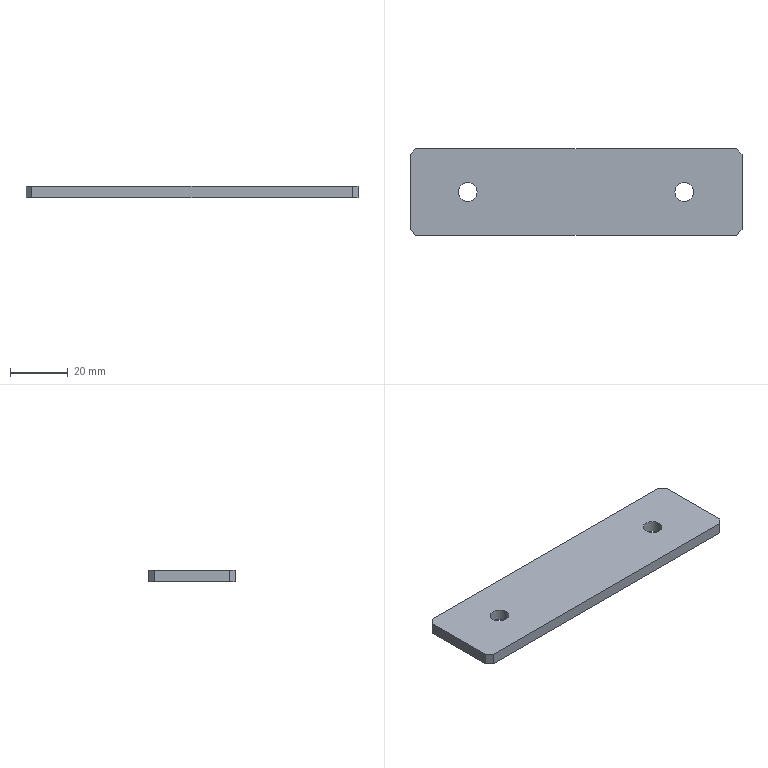Part | SolidWorks | features Chamfer 1, Extrusion 1 | 1 solid | 14 faces | box 115 x 30 x 4 mm | volume 13503 mm3 | plane 10 | cylinder 4 | commonest cylinder face diameters 6.5 x4
STEP:
#1=CARTESIAN_POINT('',(34.25,0.,4.));
#2=VERTEX_POINT('',#1);
#3=CARTESIAN_POINT('',(40.75,0.,4.));
#4=VERTEX_POINT('',#3);
#5=CARTESIAN_POINT('',(37.5,0.,4.));
#6=DIRECTION('',(0.,0.,1.));
#7=DIRECTION('',(1.,0.,0.));
#8=AXIS2_PLACEMENT_3D('',#5,#6,#7);
#9=CIRCLE('',#8,3.25);
#10=EDGE_CURVE('',#2,#4,#9,.T.);
#11=ORIENTED_EDGE('',*,*,#10,.T.);
#12=CARTESIAN_POINT('',(40.75,0.,0.));
#13=VERTEX_POINT('',#12);
#14=CARTESIAN_POINT('',(40.75,0.,4.));
#15=DIRECTION('',(0.,0.,-1.));
#16=VECTOR('',#15,1000.);
#17=LINE('',#14,#16);
#18=EDGE_CURVE('',#4,#13,#17,.T.);
#19=ORIENTED_EDGE('',*,*,#18,.T.);
#20=CARTESIAN_POINT('',(34.25,0.,0.));
#21=VERTEX_POINT('',#20);
#22=CARTESIAN_POINT('',(37.5,0.,0.));
#23=DIRECTION('',(0.,0.,1.));
#24=DIRECTION('',(1.,0.,0.));
#25=AXIS2_PLACEMENT_3D('',#22,#23,#24);
#26=CIRCLE('',#25,3.25);
#27=EDGE_CURVE('',#21,#13,#26,.T.);
#28=ORIENTED_EDGE('',*,*,#27,.F.);
#29=CARTESIAN_POINT('',(34.25,0.,4.));
#30=DIRECTION('',(0.,0.,-1.));
#31=VECTOR('',#30,1000.);
#32=LINE('',#29,#31);
#33=EDGE_CURVE('',#2,#21,#32,.T.);
#34=ORIENTED_EDGE('',*,*,#33,.F.);
#35=EDGE_LOOP('',(#11,#19,#28,#34));
#36=FACE_OUTER_BOUND('',#35,.T.);
#37=CARTESIAN_POINT('',(37.5,0.,4.));
#38=DIRECTION('',(0.,0.,-1.));
#39=DIRECTION('',(-1.,0.,0.));
#40=AXIS2_PLACEMENT_3D('',#37,#38,#39);
#41=CYLINDRICAL_SURFACE('',#40,3.25);
#42=ADVANCED_FACE('',(#36),#41,.F.);
#43=CARTESIAN_POINT('',(-40.75,0.,4.));
#44=VERTEX_POINT('',#43);
#45=CARTESIAN_POINT('',(-34.25,0.,4.));
#46=VERTEX_POINT('',#45);
#47=CARTESIAN_POINT('',(-37.5,0.,4.));
#48=DIRECTION('',(0.,0.,1.));
#49=DIRECTION('',(1.,0.,0.));
#50=AXIS2_PLACEMENT_3D('',#47,#48,#49);
#51=CIRCLE('',#50,3.25);
#52=EDGE_CURVE('',#44,#46,#51,.T.);
#53=ORIENTED_EDGE('',*,*,#52,.T.);
#54=CARTESIAN_POINT('',(-34.25,0.,0.));
#55=VERTEX_POINT('',#54);
#56=CARTESIAN_POINT('',(-34.25,0.,4.));
#57=DIRECTION('',(0.,0.,-1.));
#58=VECTOR('',#57,1000.);
#59=LINE('',#56,#58);
#60=EDGE_CURVE('',#46,#55,#59,.T.);
#61=ORIENTED_EDGE('',*,*,#60,.T.);
#62=CARTESIAN_POINT('',(-40.75,0.,0.));
#63=VERTEX_POINT('',#62);
#64=CARTESIAN_POINT('',(-37.5,0.,0.));
#65=DIRECTION('',(0.,0.,1.));
#66=DIRECTION('',(1.,0.,0.));
#67=AXIS2_PLACEMENT_3D('',#64,#65,#66);
#68=CIRCLE('',#67,3.25);
#69=EDGE_CURVE('',#63,#55,#68,.T.);
#70=ORIENTED_EDGE('',*,*,#69,.F.);
#71=CARTESIAN_POINT('',(-40.75,0.,4.));
#72=DIRECTION('',(0.,0.,-1.));
#73=VECTOR('',#72,1000.);
#74=LINE('',#71,#73);
#75=EDGE_CURVE('',#44,#63,#74,.T.);
#76=ORIENTED_EDGE('',*,*,#75,.F.);
#77=EDGE_LOOP('',(#53,#61,#70,#76));
#78=FACE_OUTER_BOUND('',#77,.T.);
#79=CARTESIAN_POINT('',(-37.5,0.,4.));
#80=DIRECTION('',(0.,0.,-1.));
#81=DIRECTION('',(-1.,0.,0.));
#82=AXIS2_PLACEMENT_3D('',#79,#80,#81);
#83=CYLINDRICAL_SURFACE('',#82,3.25);
#84=ADVANCED_FACE('',(#78),#83,.F.);
#85=CARTESIAN_POINT('',(-57.5,13.,4.));
#86=VERTEX_POINT('',#85);
#87=CARTESIAN_POINT('',(-57.5,-13.,4.));
#88=VERTEX_POINT('',#87);
#89=CARTESIAN_POINT('',(-57.5,15.,4.));
#90=DIRECTION('',(0.,-1.,0.));
#91=VECTOR('',#90,1000.);
#92=LINE('',#89,#91);
#93=EDGE_CURVE('',#86,#88,#92,.T.);
#94=ORIENTED_EDGE('',*,*,#93,.T.);
#95=CARTESIAN_POINT('',(-55.5,-15.,4.));
#96=VERTEX_POINT('',#95);
#97=CARTESIAN_POINT('',(-55.5,-15.,4.));
#98=DIRECTION('',(0.7071,-0.7071,0.));
#99=VECTOR('',#98,1000.);
#100=LINE('',#97,#99);
#101=EDGE_CURVE('',#88,#96,#100,.T.);
#102=ORIENTED_EDGE('',*,*,#101,.T.);
#103=CARTESIAN_POINT('',(55.5,-15.,4.));
#104=VERTEX_POINT('',#103);
#105=CARTESIAN_POINT('',(57.5,-15.,4.));
#106=DIRECTION('',(1.,0.,0.));
#107=VECTOR('',#106,1000.);
#108=LINE('',#105,#107);
#109=EDGE_CURVE('',#96,#104,#108,.T.);
#110=ORIENTED_EDGE('',*,*,#109,.T.);
#111=CARTESIAN_POINT('',(57.5,-13.,4.));
#112=VERTEX_POINT('',#111);
#113=CARTESIAN_POINT('',(57.5,-13.,4.));
#114=DIRECTION('',(0.7071,0.7071,0.));
#115=VECTOR('',#114,1000.);
#116=LINE('',#113,#115);
#117=EDGE_CURVE('',#104,#112,#116,.T.);
#118=ORIENTED_EDGE('',*,*,#117,.T.);
#119=CARTESIAN_POINT('',(57.5,13.,4.));
#120=VERTEX_POINT('',#119);
#121=CARTESIAN_POINT('',(57.5,15.,4.));
#122=DIRECTION('',(0.,1.,0.));
#123=VECTOR('',#122,1000.);
#124=LINE('',#121,#123);
#125=EDGE_CURVE('',#112,#120,#124,.T.);
#126=ORIENTED_EDGE('',*,*,#125,.T.);
#127=CARTESIAN_POINT('',(55.5,15.,4.));
#128=VERTEX_POINT('',#127);
#129=CARTESIAN_POINT('',(55.5,15.,4.));
#130=DIRECTION('',(-0.7071,0.7071,0.));
#131=VECTOR('',#130,1000.);
#132=LINE('',#129,#131);
#133=EDGE_CURVE('',#120,#128,#132,.T.);
#134=ORIENTED_EDGE('',*,*,#133,.T.);
#135=CARTESIAN_POINT('',(-55.5,15.,4.));
#136=VERTEX_POINT('',#135);
#137=CARTESIAN_POINT('',(57.5,15.,4.));
#138=DIRECTION('',(-1.,0.,0.));
#139=VECTOR('',#138,1000.);
#140=LINE('',#137,#139);
#141=EDGE_CURVE('',#128,#136,#140,.T.);
#142=ORIENTED_EDGE('',*,*,#141,.T.);
#143=CARTESIAN_POINT('',(-57.5,13.,4.));
#144=DIRECTION('',(-0.7071,-0.7071,0.));
#145=VECTOR('',#144,1000.);
#146=LINE('',#143,#145);
#147=EDGE_CURVE('',#136,#86,#146,.T.);
#148=ORIENTED_EDGE('',*,*,#147,.T.);
#149=EDGE_LOOP('',(#94,#102,#110,#118,#126,#134,#142,#148));
#150=FACE_OUTER_BOUND('',#149,.T.);
#151=ORIENTED_EDGE('',*,*,#52,.F.);
#152=CARTESIAN_POINT('',(-37.5,0.,4.));
#153=DIRECTION('',(0.,0.,1.));
#154=DIRECTION('',(1.,0.,0.));
#155=AXIS2_PLACEMENT_3D('',#152,#153,#154);
#156=CIRCLE('',#155,3.25);
#157=EDGE_CURVE('',#46,#44,#156,.T.);
#158=ORIENTED_EDGE('',*,*,#157,.F.);
#159=EDGE_LOOP('',(#151,#158));
#160=FACE_BOUND('',#159,.T.);
#161=ORIENTED_EDGE('',*,*,#10,.F.);
#162=CARTESIAN_POINT('',(37.5,0.,4.));
#163=DIRECTION('',(0.,0.,1.));
#164=DIRECTION('',(1.,0.,0.));
#165=AXIS2_PLACEMENT_3D('',#162,#163,#164);
#166=CIRCLE('',#165,3.25);
#167=EDGE_CURVE('',#4,#2,#166,.T.);
#168=ORIENTED_EDGE('',*,*,#167,.F.);
#169=EDGE_LOOP('',(#161,#168));
#170=FACE_BOUND('',#169,.T.);
#171=CARTESIAN_POINT('',(0.,0.,4.));
#172=DIRECTION('',(0.,0.,-1.));
#173=DIRECTION('',(-1.,0.,0.));
#174=AXIS2_PLACEMENT_3D('',#171,#172,#173);
#175=PLANE('',#174);
#176=ADVANCED_FACE('',(#150,#160,#170),#175,.F.);
#177=ORIENTED_EDGE('',*,*,#69,.T.);
#178=CARTESIAN_POINT('',(-37.5,0.,0.));
#179=DIRECTION('',(0.,0.,1.));
#180=DIRECTION('',(1.,0.,0.));
#181=AXIS2_PLACEMENT_3D('',#178,#179,#180);
#182=CIRCLE('',#181,3.25);
#183=EDGE_CURVE('',#55,#63,#182,.T.);
#184=ORIENTED_EDGE('',*,*,#183,.T.);
#185=EDGE_LOOP('',(#177,#184));
#186=FACE_BOUND('',#185,.T.);
#187=CARTESIAN_POINT('',(-55.5,-15.,0.));
#188=VERTEX_POINT('',#187);
#189=CARTESIAN_POINT('',(55.5,-15.,0.));
#190=VERTEX_POINT('',#189);
#191=CARTESIAN_POINT('',(57.5,-15.,0.));
#192=DIRECTION('',(1.,0.,0.));
#193=VECTOR('',#192,1000.);
#194=LINE('',#191,#193);
#195=EDGE_CURVE('',#188,#190,#194,.T.);
#196=ORIENTED_EDGE('',*,*,#195,.F.);
#197=CARTESIAN_POINT('',(-57.5,-13.,0.));
#198=VERTEX_POINT('',#197);
#199=CARTESIAN_POINT('',(-35.25,-35.25,0.));
#200=DIRECTION('',(-0.7071,0.7071,0.));
#201=VECTOR('',#200,1000.);
#202=LINE('',#199,#201);
#203=EDGE_CURVE('',#188,#198,#202,.T.);
#204=ORIENTED_EDGE('',*,*,#203,.T.);
#205=CARTESIAN_POINT('',(-57.5,13.,0.));
#206=VERTEX_POINT('',#205);
#207=CARTESIAN_POINT('',(-57.5,15.,0.));
#208=DIRECTION('',(0.,-1.,0.));
#209=VECTOR('',#208,1000.);
#210=LINE('',#207,#209);
#211=EDGE_CURVE('',#206,#198,#210,.T.);
#212=ORIENTED_EDGE('',*,*,#211,.F.);
#213=CARTESIAN_POINT('',(-55.5,15.,0.));
#214=VERTEX_POINT('',#213);
#215=CARTESIAN_POINT('',(-35.25,35.25,0.));
#216=DIRECTION('',(0.7071,0.7071,0.));
#217=VECTOR('',#216,1000.);
#218=LINE('',#215,#217);
#219=EDGE_CURVE('',#206,#214,#218,.T.);
#220=ORIENTED_EDGE('',*,*,#219,.T.);
#221=CARTESIAN_POINT('',(55.5,15.,0.));
#222=VERTEX_POINT('',#221);
#223=CARTESIAN_POINT('',(57.5,15.,0.));
#224=DIRECTION('',(-1.,0.,0.));
#225=VECTOR('',#224,1000.);
#226=LINE('',#223,#225);
#227=EDGE_CURVE('',#222,#214,#226,.T.);
#228=ORIENTED_EDGE('',*,*,#227,.F.);
#229=CARTESIAN_POINT('',(57.5,13.,0.));
#230=VERTEX_POINT('',#229);
#231=CARTESIAN_POINT('',(35.25,35.25,0.));
#232=DIRECTION('',(0.7071,-0.7071,0.));
#233=VECTOR('',#232,1000.);
#234=LINE('',#231,#233);
#235=EDGE_CURVE('',#222,#230,#234,.T.);
#236=ORIENTED_EDGE('',*,*,#235,.T.);
#237=CARTESIAN_POINT('',(57.5,-13.,0.));
#238=VERTEX_POINT('',#237);
#239=CARTESIAN_POINT('',(57.5,15.,0.));
#240=DIRECTION('',(0.,1.,0.));
#241=VECTOR('',#240,1000.);
#242=LINE('',#239,#241);
#243=EDGE_CURVE('',#238,#230,#242,.T.);
#244=ORIENTED_EDGE('',*,*,#243,.F.);
#245=CARTESIAN_POINT('',(35.25,-35.25,0.));
#246=DIRECTION('',(-0.7071,-0.7071,0.));
#247=VECTOR('',#246,1000.);
#248=LINE('',#245,#247);
#249=EDGE_CURVE('',#238,#190,#248,.T.);
#250=ORIENTED_EDGE('',*,*,#249,.T.);
#251=EDGE_LOOP('',(#196,#204,#212,#220,#228,#236,#244,#250));
#252=FACE_OUTER_BOUND('',#251,.T.);
#253=ORIENTED_EDGE('',*,*,#27,.T.);
#254=CARTESIAN_POINT('',(37.5,0.,0.));
#255=DIRECTION('',(0.,0.,1.));
#256=DIRECTION('',(1.,0.,0.));
#257=AXIS2_PLACEMENT_3D('',#254,#255,#256);
#258=CIRCLE('',#257,3.25);
#259=EDGE_CURVE('',#13,#21,#258,.T.);
#260=ORIENTED_EDGE('',*,*,#259,.T.);
#261=EDGE_LOOP('',(#253,#260));
#262=FACE_BOUND('',#261,.T.);
#263=CARTESIAN_POINT('',(0.,0.,0.));
#264=DIRECTION('',(0.,0.,-1.));
#265=DIRECTION('',(-1.,0.,0.));
#266=AXIS2_PLACEMENT_3D('',#263,#264,#265);
#267=PLANE('',#266);
#268=ADVANCED_FACE('',(#186,#252,#262),#267,.T.);
#269=ORIENTED_EDGE('',*,*,#211,.T.);
#270=CARTESIAN_POINT('',(-57.5,-13.,4.));
#271=DIRECTION('',(0.,0.,1.));
#272=VECTOR('',#271,1000.);
#273=LINE('',#270,#272);
#274=EDGE_CURVE('',#198,#88,#273,.T.);
#275=ORIENTED_EDGE('',*,*,#274,.T.);
#276=ORIENTED_EDGE('',*,*,#93,.F.);
#277=CARTESIAN_POINT('',(-57.5,13.,4.));
#278=DIRECTION('',(0.,0.,-1.));
#279=VECTOR('',#278,1000.);
#280=LINE('',#277,#279);
#281=EDGE_CURVE('',#86,#206,#280,.T.);
#282=ORIENTED_EDGE('',*,*,#281,.T.);
#283=EDGE_LOOP('',(#269,#275,#276,#282));
#284=FACE_OUTER_BOUND('',#283,.T.);
#285=CARTESIAN_POINT('',(-57.5,15.,4.));
#286=DIRECTION('',(1.,0.,0.));
#287=DIRECTION('',(0.,0.,-1.));
#288=AXIS2_PLACEMENT_3D('',#285,#286,#287);
#289=PLANE('',#288);
#290=ADVANCED_FACE('',(#284),#289,.F.);
#291=ORIENTED_EDGE('',*,*,#109,.F.);
#292=CARTESIAN_POINT('',(-55.5,-15.,4.));
#293=DIRECTION('',(0.,0.,-1.));
#294=VECTOR('',#293,1000.);
#295=LINE('',#292,#294);
#296=EDGE_CURVE('',#96,#188,#295,.T.);
#297=ORIENTED_EDGE('',*,*,#296,.T.);
#298=ORIENTED_EDGE('',*,*,#195,.T.);
#299=CARTESIAN_POINT('',(55.5,-15.,4.));
#300=DIRECTION('',(0.,0.,1.));
#301=VECTOR('',#300,1000.);
#302=LINE('',#299,#301);
#303=EDGE_CURVE('',#190,#104,#302,.T.);
#304=ORIENTED_EDGE('',*,*,#303,.T.);
#305=EDGE_LOOP('',(#291,#297,#298,#304));
#306=FACE_OUTER_BOUND('',#305,.T.);
#307=CARTESIAN_POINT('',(57.5,-15.,4.));
#308=DIRECTION('',(0.,1.,0.));
#309=DIRECTION('',(-1.,0.,0.));
#310=AXIS2_PLACEMENT_3D('',#307,#308,#309);
#311=PLANE('',#310);
#312=ADVANCED_FACE('',(#306),#311,.F.);
#313=ORIENTED_EDGE('',*,*,#125,.F.);
#314=CARTESIAN_POINT('',(57.5,-13.,4.));
#315=DIRECTION('',(0.,0.,-1.));
#316=VECTOR('',#315,1000.);
#317=LINE('',#314,#316);
#318=EDGE_CURVE('',#112,#238,#317,.T.);
#319=ORIENTED_EDGE('',*,*,#318,.T.);
#320=ORIENTED_EDGE('',*,*,#243,.T.);
#321=CARTESIAN_POINT('',(57.5,13.,4.));
#322=DIRECTION('',(0.,0.,1.));
#323=VECTOR('',#322,1000.);
#324=LINE('',#321,#323);
#325=EDGE_CURVE('',#230,#120,#324,.T.);
#326=ORIENTED_EDGE('',*,*,#325,.T.);
#327=EDGE_LOOP('',(#313,#319,#320,#326));
#328=FACE_OUTER_BOUND('',#327,.T.);
#329=CARTESIAN_POINT('',(57.5,15.,4.));
#330=DIRECTION('',(-1.,0.,0.));
#331=DIRECTION('',(0.,-1.,0.));
#332=AXIS2_PLACEMENT_3D('',#329,#330,#331);
#333=PLANE('',#332);
#334=ADVANCED_FACE('',(#328),#333,.F.);
#335=ORIENTED_EDGE('',*,*,#227,.T.);
#336=CARTESIAN_POINT('',(-55.5,15.,4.));
#337=DIRECTION('',(0.,0.,1.));
#338=VECTOR('',#337,1000.);
#339=LINE('',#336,#338);
#340=EDGE_CURVE('',#214,#136,#339,.T.);
#341=ORIENTED_EDGE('',*,*,#340,.T.);
#342=ORIENTED_EDGE('',*,*,#141,.F.);
#343=CARTESIAN_POINT('',(55.5,15.,4.));
#344=DIRECTION('',(0.,0.,-1.));
#345=VECTOR('',#344,1000.);
#346=LINE('',#343,#345);
#347=EDGE_CURVE('',#128,#222,#346,.T.);
#348=ORIENTED_EDGE('',*,*,#347,.T.);
#349=EDGE_LOOP('',(#335,#341,#342,#348));
#350=FACE_OUTER_BOUND('',#349,.T.);
#351=CARTESIAN_POINT('',(57.5,15.,4.));
#352=DIRECTION('',(0.,-1.,0.));
#353=DIRECTION('',(1.,0.,0.));
#354=AXIS2_PLACEMENT_3D('',#351,#352,#353);
#355=PLANE('',#354);
#356=ADVANCED_FACE('',(#350),#355,.F.);
#357=ORIENTED_EDGE('',*,*,#60,.F.);
#358=ORIENTED_EDGE('',*,*,#157,.T.);
#359=ORIENTED_EDGE('',*,*,#75,.T.);
#360=ORIENTED_EDGE('',*,*,#183,.F.);
#361=EDGE_LOOP('',(#357,#358,#359,#360));
#362=FACE_OUTER_BOUND('',#361,.T.);
#363=CARTESIAN_POINT('',(-37.5,0.,4.));
#364=DIRECTION('',(0.,0.,-1.));
#365=DIRECTION('',(-1.,0.,0.));
#366=AXIS2_PLACEMENT_3D('',#363,#364,#365);
#367=CYLINDRICAL_SURFACE('',#366,3.25);
#368=ADVANCED_FACE('',(#362),#367,.F.);
#369=ORIENTED_EDGE('',*,*,#18,.F.);
#370=ORIENTED_EDGE('',*,*,#167,.T.);
#371=ORIENTED_EDGE('',*,*,#33,.T.);
#372=ORIENTED_EDGE('',*,*,#259,.F.);
#373=EDGE_LOOP('',(#369,#370,#371,#372));
#374=FACE_OUTER_BOUND('',#373,.T.);
#375=CARTESIAN_POINT('',(37.5,0.,4.));
#376=DIRECTION('',(0.,0.,-1.));
#377=DIRECTION('',(-1.,0.,0.));
#378=AXIS2_PLACEMENT_3D('',#375,#376,#377);
#379=CYLINDRICAL_SURFACE('',#378,3.25);
#380=ADVANCED_FACE('',(#374),#379,.F.);
#381=ORIENTED_EDGE('',*,*,#101,.F.);
#382=ORIENTED_EDGE('',*,*,#274,.F.);
#383=ORIENTED_EDGE('',*,*,#203,.F.);
#384=ORIENTED_EDGE('',*,*,#296,.F.);
#385=EDGE_LOOP('',(#381,#382,#383,#384));
#386=FACE_OUTER_BOUND('',#385,.T.);
#387=CARTESIAN_POINT('',(-55.5,-15.,4.));
#388=DIRECTION('',(0.7071,0.7071,0.));
#389=DIRECTION('',(0.,0.,-1.));
#390=AXIS2_PLACEMENT_3D('',#387,#388,#389);
#391=PLANE('',#390);
#392=ADVANCED_FACE('',(#386),#391,.F.);
#393=ORIENTED_EDGE('',*,*,#147,.F.);
#394=ORIENTED_EDGE('',*,*,#340,.F.);
#395=ORIENTED_EDGE('',*,*,#219,.F.);
#396=ORIENTED_EDGE('',*,*,#281,.F.);
#397=EDGE_LOOP('',(#393,#394,#395,#396));
#398=FACE_OUTER_BOUND('',#397,.T.);
#399=CARTESIAN_POINT('',(-57.5,13.,4.));
#400=DIRECTION('',(0.7071,-0.7071,0.));
#401=DIRECTION('',(0.,0.,-1.));
#402=AXIS2_PLACEMENT_3D('',#399,#400,#401);
#403=PLANE('',#402);
#404=ADVANCED_FACE('',(#398),#403,.F.);
#405=ORIENTED_EDGE('',*,*,#117,.F.);
#406=ORIENTED_EDGE('',*,*,#303,.F.);
#407=ORIENTED_EDGE('',*,*,#249,.F.);
#408=ORIENTED_EDGE('',*,*,#318,.F.);
#409=EDGE_LOOP('',(#405,#406,#407,#408));
#410=FACE_OUTER_BOUND('',#409,.T.);
#411=CARTESIAN_POINT('',(57.5,-13.,4.));
#412=DIRECTION('',(-0.7071,0.7071,0.));
#413=DIRECTION('',(0.,0.,-1.));
#414=AXIS2_PLACEMENT_3D('',#411,#412,#413);
#415=PLANE('',#414);
#416=ADVANCED_FACE('',(#410),#415,.F.);
#417=ORIENTED_EDGE('',*,*,#133,.F.);
#418=ORIENTED_EDGE('',*,*,#325,.F.);
#419=ORIENTED_EDGE('',*,*,#235,.F.);
#420=ORIENTED_EDGE('',*,*,#347,.F.);
#421=EDGE_LOOP('',(#417,#418,#419,#420));
#422=FACE_OUTER_BOUND('',#421,.T.);
#423=CARTESIAN_POINT('',(55.5,15.,4.));
#424=DIRECTION('',(-0.7071,-0.7071,0.));
#425=DIRECTION('',(0.,0.,-1.));
#426=AXIS2_PLACEMENT_3D('',#423,#424,#425);
#427=PLANE('',#426);
#428=ADVANCED_FACE('',(#422),#427,.F.);
#429=CLOSED_SHELL('',(#42,#84,#176,#268,#290,#312,#334,#356,#368,#380,#392,#404,#416,#428));
#430=MANIFOLD_SOLID_BREP('',#429);
#431=CARTESIAN_POINT('',(0.,0.,0.));
#432=DIRECTION('',(0.,0.,1.));
#433=DIRECTION('',(1.,0.,0.));
#434=AXIS2_PLACEMENT_3D('',#431,#432,#433);
#435=(LENGTH_UNIT()NAMED_UNIT(*)SI_UNIT(.MILLI.,.METRE.));
#436=UNCERTAINTY_MEASURE_WITH_UNIT(LENGTH_MEASURE(0.00001),#435,'','');
#437=(NAMED_UNIT(*)PLANE_ANGLE_UNIT()SI_UNIT($,.RADIAN.));
#438=(NAMED_UNIT(*)SI_UNIT($,.STERADIAN.)SOLID_ANGLE_UNIT());
#439=(GEOMETRIC_REPRESENTATION_CONTEXT(3)GLOBAL_UNCERTAINTY_ASSIGNED_CONTEXT((#436))GLOBAL_UNIT_ASSIGNED_CONTEXT((#435,#437,#438))REPRESENTATION_CONTEXT('',''));
#440=ADVANCED_BREP_SHAPE_REPRESENTATION('',(#430,#434),#439);